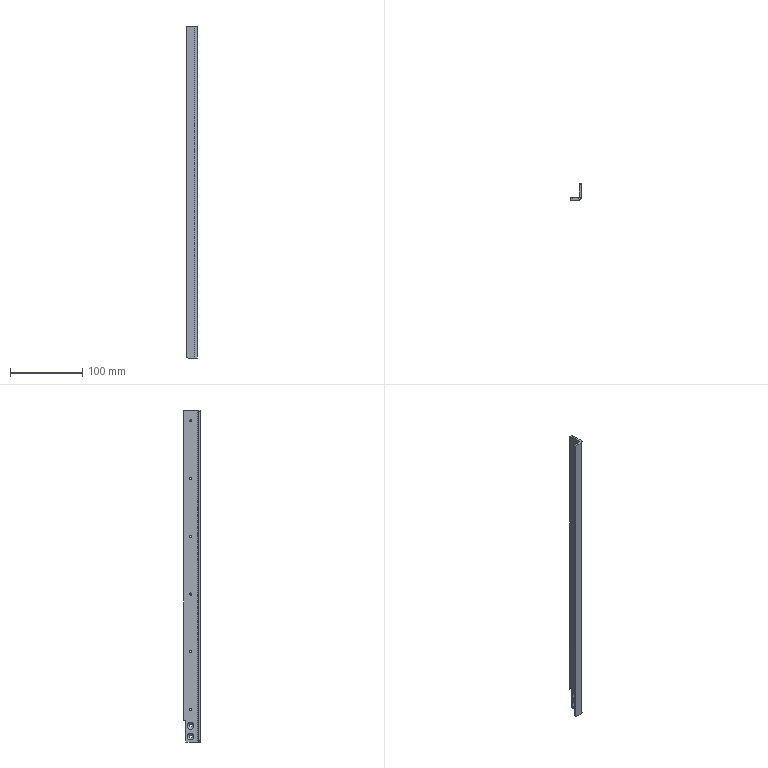Part | NX | features BREP 1 | 1 solid | 51 faces | box 15 x 23 x 460 mm | volume 46240 mm3 | cylinder 21 | cone 16 | plane 14 | commonest cylinder face diameters 2.5 x12 4.5 x4 4 x3 2 x1 8 x1
STEP:
#1=CARTESIAN_POINT('',(-12.,-3.,-228.));
#2=VERTEX_POINT('',#1);
#3=CARTESIAN_POINT('',(-10.,-3.,-230.));
#4=VERTEX_POINT('',#3);
#5=CARTESIAN_POINT('',(-10.,-3.,-228.));
#6=DIRECTION('',(0.,-1.,0.));
#7=DIRECTION('',(-1.,0.,0.));
#8=AXIS2_PLACEMENT_3D('',#5,#6,#7);
#9=CIRCLE('',#8,2.);
#10=EDGE_CURVE('',#2,#4,#9,.T.);
#11=ORIENTED_EDGE('',*,*,#10,.F.);
#12=CARTESIAN_POINT('',(-12.,0.,-228.));
#13=VERTEX_POINT('',#12);
#14=CARTESIAN_POINT('',(-12.,-3.,-228.));
#15=DIRECTION('',(0.,-1.,0.));
#16=VECTOR('',#15,1000.);
#17=LINE('',#14,#16);
#18=EDGE_CURVE('',#13,#2,#17,.T.);
#19=ORIENTED_EDGE('',*,*,#18,.F.);
#20=CARTESIAN_POINT('',(-10.,0.,-230.));
#21=VERTEX_POINT('',#20);
#22=CARTESIAN_POINT('',(-10.,0.,-228.));
#23=DIRECTION('',(0.,1.,0.));
#24=DIRECTION('',(-1.,0.,0.));
#25=AXIS2_PLACEMENT_3D('',#22,#23,#24);
#26=CIRCLE('',#25,2.);
#27=EDGE_CURVE('',#21,#13,#26,.T.);
#28=ORIENTED_EDGE('',*,*,#27,.F.);
#29=CARTESIAN_POINT('',(-10.,1.,-230.));
#30=DIRECTION('',(0.,1.,0.));
#31=VECTOR('',#30,1000.);
#32=LINE('',#29,#31);
#33=EDGE_CURVE('',#4,#21,#32,.T.);
#34=ORIENTED_EDGE('',*,*,#33,.F.);
#35=EDGE_LOOP('',(#11,#19,#28,#34));
#36=FACE_BOUND('',#35,.T.);
#37=CARTESIAN_POINT('',(-10.,1.,-228.));
#38=DIRECTION('',(0.,1.,0.));
#39=DIRECTION('',(0.,0.,1.));
#40=AXIS2_PLACEMENT_3D('',#37,#38,#39);
#41=CYLINDRICAL_SURFACE('',#40,2.);
#42=ADVANCED_FACE('',(#36),#41,.T.);
#43=CARTESIAN_POINT('',(-10.,-3.,230.));
#44=VERTEX_POINT('',#43);
#45=CARTESIAN_POINT('',(-12.,-3.,228.));
#46=VERTEX_POINT('',#45);
#47=CARTESIAN_POINT('',(-10.,-3.,228.));
#48=DIRECTION('',(0.,-1.,0.));
#49=DIRECTION('',(-1.,0.,0.));
#50=AXIS2_PLACEMENT_3D('',#47,#48,#49);
#51=CIRCLE('',#50,2.);
#52=EDGE_CURVE('',#44,#46,#51,.T.);
#53=ORIENTED_EDGE('',*,*,#52,.F.);
#54=CARTESIAN_POINT('',(-10.,0.,230.));
#55=VERTEX_POINT('',#54);
#56=CARTESIAN_POINT('',(-10.,-3.,230.));
#57=DIRECTION('',(0.,-1.,0.));
#58=VECTOR('',#57,1000.);
#59=LINE('',#56,#58);
#60=EDGE_CURVE('',#55,#44,#59,.T.);
#61=ORIENTED_EDGE('',*,*,#60,.F.);
#62=CARTESIAN_POINT('',(-12.,0.,228.));
#63=VERTEX_POINT('',#62);
#64=CARTESIAN_POINT('',(-10.,0.,228.));
#65=DIRECTION('',(0.,1.,0.));
#66=DIRECTION('',(-1.,0.,0.));
#67=AXIS2_PLACEMENT_3D('',#64,#65,#66);
#68=CIRCLE('',#67,2.);
#69=EDGE_CURVE('',#63,#55,#68,.T.);
#70=ORIENTED_EDGE('',*,*,#69,.F.);
#71=CARTESIAN_POINT('',(-12.,0.,228.));
#72=DIRECTION('',(0.,1.,0.));
#73=VECTOR('',#72,1000.);
#74=LINE('',#71,#73);
#75=EDGE_CURVE('',#46,#63,#74,.T.);
#76=ORIENTED_EDGE('',*,*,#75,.F.);
#77=EDGE_LOOP('',(#53,#61,#70,#76));
#78=FACE_BOUND('',#77,.T.);
#79=CARTESIAN_POINT('',(-10.,-3.,228.));
#80=DIRECTION('',(0.,-1.,0.));
#81=DIRECTION('',(0.,0.,-1.));
#82=AXIS2_PLACEMENT_3D('',#79,#80,#81);
#83=CYLINDRICAL_SURFACE('',#82,2.);
#84=ADVANCED_FACE('',(#78),#83,.T.);
#85=CARTESIAN_POINT('',(0.,18.,230.));
#86=VERTEX_POINT('',#85);
#87=CARTESIAN_POINT('',(0.,20.,228.));
#88=VERTEX_POINT('',#87);
#89=CARTESIAN_POINT('',(0.,18.,228.));
#90=DIRECTION('',(-1.,0.,0.));
#91=DIRECTION('',(0.,0.,1.));
#92=AXIS2_PLACEMENT_3D('',#89,#90,#91);
#93=CIRCLE('',#92,2.);
#94=EDGE_CURVE('',#86,#88,#93,.T.);
#95=ORIENTED_EDGE('',*,*,#94,.F.);
#96=CARTESIAN_POINT('',(3.,18.,230.));
#97=VERTEX_POINT('',#96);
#98=CARTESIAN_POINT('',(-1.,18.,230.));
#99=DIRECTION('',(-1.,0.,0.));
#100=VECTOR('',#99,1000.);
#101=LINE('',#98,#100);
#102=EDGE_CURVE('',#97,#86,#101,.T.);
#103=ORIENTED_EDGE('',*,*,#102,.F.);
#104=CARTESIAN_POINT('',(3.,20.,228.));
#105=VERTEX_POINT('',#104);
#106=CARTESIAN_POINT('',(3.,18.,228.));
#107=DIRECTION('',(1.,0.,0.));
#108=DIRECTION('',(0.,0.,1.));
#109=AXIS2_PLACEMENT_3D('',#106,#107,#108);
#110=CIRCLE('',#109,2.);
#111=EDGE_CURVE('',#105,#97,#110,.T.);
#112=ORIENTED_EDGE('',*,*,#111,.F.);
#113=CARTESIAN_POINT('',(0.,20.,228.));
#114=DIRECTION('',(1.,0.,0.));
#115=VECTOR('',#114,1000.);
#116=LINE('',#113,#115);
#117=EDGE_CURVE('',#88,#105,#116,.T.);
#118=ORIENTED_EDGE('',*,*,#117,.F.);
#119=EDGE_LOOP('',(#95,#103,#112,#118));
#120=FACE_BOUND('',#119,.T.);
#121=CARTESIAN_POINT('',(0.,18.,228.));
#122=DIRECTION('',(1.,0.,0.));
#123=DIRECTION('',(0.,0.,-1.));
#124=AXIS2_PLACEMENT_3D('',#121,#122,#123);
#125=CYLINDRICAL_SURFACE('',#124,2.);
#126=ADVANCED_FACE('',(#120),#125,.T.);
#127=CARTESIAN_POINT('',(0.,10.5,213.475));
#128=VERTEX_POINT('',#127);
#129=CARTESIAN_POINT('',(0.275,10.5,213.75));
#130=VERTEX_POINT('',#129);
#131=CARTESIAN_POINT('',(0.,10.5,213.475));
#132=DIRECTION('',(-0.7071,0.,-0.7071));
#133=VECTOR('',#132,1000.);
#134=LINE('',#131,#133);
#135=EDGE_CURVE('',#128,#130,#134,.F.);
#136=ORIENTED_EDGE('',*,*,#135,.T.);
#137=CARTESIAN_POINT('',(0.275,10.5,216.25));
#138=VERTEX_POINT('',#137);
#139=CARTESIAN_POINT('',(0.275,10.5,215.));
#140=DIRECTION('',(-1.,0.,0.));
#141=DIRECTION('',(0.,0.,1.));
#142=AXIS2_PLACEMENT_3D('',#139,#140,#141);
#143=CIRCLE('',#142,1.25);
#144=EDGE_CURVE('',#138,#130,#143,.T.);
#145=ORIENTED_EDGE('',*,*,#144,.F.);
#146=CARTESIAN_POINT('',(0.,10.5,216.525));
#147=VERTEX_POINT('',#146);
#148=CARTESIAN_POINT('',(0.,10.5,216.525));
#149=DIRECTION('',(-0.7071,0.,0.7071));
#150=VECTOR('',#149,1000.);
#151=LINE('',#148,#150);
#152=EDGE_CURVE('',#147,#138,#151,.F.);
#153=ORIENTED_EDGE('',*,*,#152,.F.);
#154=CARTESIAN_POINT('',(0.,10.5,215.));
#155=DIRECTION('',(-1.,0.,0.));
#156=DIRECTION('',(0.,0.,1.));
#157=AXIS2_PLACEMENT_3D('',#154,#155,#156);
#158=CIRCLE('',#157,1.525);
#159=EDGE_CURVE('',#147,#128,#158,.T.);
#160=ORIENTED_EDGE('',*,*,#159,.T.);
#161=EDGE_LOOP('',(#136,#145,#153,#160));
#162=FACE_BOUND('',#161,.T.);
#163=CARTESIAN_POINT('',(0.,10.5,215.));
#164=DIRECTION('',(-1.,0.,0.));
#165=DIRECTION('',(0.,0.,1.));
#166=AXIS2_PLACEMENT_3D('',#163,#164,#165);
#167=CONICAL_SURFACE('',#166,1.525,0.7854);
#168=ADVANCED_FACE('',(#162),#167,.F.);
#169=CARTESIAN_POINT('',(3.,10.5,213.75));
#170=VERTEX_POINT('',#169);
#171=CARTESIAN_POINT('',(0.,10.5,213.75));
#172=DIRECTION('',(-1.,0.,0.));
#173=VECTOR('',#172,1000.);
#174=LINE('',#171,#173);
#175=EDGE_CURVE('',#130,#170,#174,.F.);
#176=ORIENTED_EDGE('',*,*,#175,.T.);
#177=CARTESIAN_POINT('',(3.,10.5,216.25));
#178=VERTEX_POINT('',#177);
#179=CARTESIAN_POINT('',(3.,10.5,215.));
#180=DIRECTION('',(-1.,0.,0.));
#181=DIRECTION('',(0.,0.,1.));
#182=AXIS2_PLACEMENT_3D('',#179,#180,#181);
#183=CIRCLE('',#182,1.25);
#184=EDGE_CURVE('',#178,#170,#183,.T.);
#185=ORIENTED_EDGE('',*,*,#184,.F.);
#186=CARTESIAN_POINT('',(0.,10.5,216.25));
#187=DIRECTION('',(-1.,0.,0.));
#188=VECTOR('',#187,1000.);
#189=LINE('',#186,#188);
#190=EDGE_CURVE('',#138,#178,#189,.F.);
#191=ORIENTED_EDGE('',*,*,#190,.F.);
#192=ORIENTED_EDGE('',*,*,#144,.T.);
#193=EDGE_LOOP('',(#176,#185,#191,#192));
#194=FACE_BOUND('',#193,.T.);
#195=CARTESIAN_POINT('',(0.,10.5,215.));
#196=DIRECTION('',(-1.,0.,0.));
#197=DIRECTION('',(0.,0.,1.));
#198=AXIS2_PLACEMENT_3D('',#195,#196,#197);
#199=CYLINDRICAL_SURFACE('',#198,1.25);
#200=ADVANCED_FACE('',(#194),#199,.F.);
#201=CARTESIAN_POINT('',(0.,10.5,133.475));
#202=VERTEX_POINT('',#201);
#203=CARTESIAN_POINT('',(0.275,10.5,133.75));
#204=VERTEX_POINT('',#203);
#205=CARTESIAN_POINT('',(0.,10.5,133.475));
#206=DIRECTION('',(-0.7071,0.,-0.7071));
#207=VECTOR('',#206,1000.);
#208=LINE('',#205,#207);
#209=EDGE_CURVE('',#202,#204,#208,.F.);
#210=ORIENTED_EDGE('',*,*,#209,.T.);
#211=CARTESIAN_POINT('',(0.275,10.5,136.25));
#212=VERTEX_POINT('',#211);
#213=CARTESIAN_POINT('',(0.275,10.5,135.));
#214=DIRECTION('',(-1.,0.,0.));
#215=DIRECTION('',(0.,0.,1.));
#216=AXIS2_PLACEMENT_3D('',#213,#214,#215);
#217=CIRCLE('',#216,1.25);
#218=EDGE_CURVE('',#212,#204,#217,.T.);
#219=ORIENTED_EDGE('',*,*,#218,.F.);
#220=CARTESIAN_POINT('',(0.,10.5,136.525));
#221=VERTEX_POINT('',#220);
#222=CARTESIAN_POINT('',(0.,10.5,136.525));
#223=DIRECTION('',(-0.7071,0.,0.7071));
#224=VECTOR('',#223,1000.);
#225=LINE('',#222,#224);
#226=EDGE_CURVE('',#221,#212,#225,.F.);
#227=ORIENTED_EDGE('',*,*,#226,.F.);
#228=CARTESIAN_POINT('',(0.,10.5,135.));
#229=DIRECTION('',(-1.,0.,0.));
#230=DIRECTION('',(0.,0.,1.));
#231=AXIS2_PLACEMENT_3D('',#228,#229,#230);
#232=CIRCLE('',#231,1.525);
#233=EDGE_CURVE('',#221,#202,#232,.T.);
#234=ORIENTED_EDGE('',*,*,#233,.T.);
#235=EDGE_LOOP('',(#210,#219,#227,#234));
#236=FACE_BOUND('',#235,.T.);
#237=CARTESIAN_POINT('',(0.,10.5,135.));
#238=DIRECTION('',(-1.,0.,0.));
#239=DIRECTION('',(0.,0.,1.));
#240=AXIS2_PLACEMENT_3D('',#237,#238,#239);
#241=CONICAL_SURFACE('',#240,1.525,0.7854);
#242=ADVANCED_FACE('',(#236),#241,.F.);
#243=CARTESIAN_POINT('',(3.,10.5,133.75));
#244=VERTEX_POINT('',#243);
#245=CARTESIAN_POINT('',(0.,10.5,133.75));
#246=DIRECTION('',(-1.,0.,0.));
#247=VECTOR('',#246,1000.);
#248=LINE('',#245,#247);
#249=EDGE_CURVE('',#204,#244,#248,.F.);
#250=ORIENTED_EDGE('',*,*,#249,.T.);
#251=CARTESIAN_POINT('',(3.,10.5,136.25));
#252=VERTEX_POINT('',#251);
#253=CARTESIAN_POINT('',(3.,10.5,135.));
#254=DIRECTION('',(-1.,0.,0.));
#255=DIRECTION('',(0.,0.,1.));
#256=AXIS2_PLACEMENT_3D('',#253,#254,#255);
#257=CIRCLE('',#256,1.25);
#258=EDGE_CURVE('',#252,#244,#257,.T.);
#259=ORIENTED_EDGE('',*,*,#258,.F.);
#260=CARTESIAN_POINT('',(0.,10.5,136.25));
#261=DIRECTION('',(-1.,0.,0.));
#262=VECTOR('',#261,1000.);
#263=LINE('',#260,#262);
#264=EDGE_CURVE('',#212,#252,#263,.F.);
#265=ORIENTED_EDGE('',*,*,#264,.F.);
#266=ORIENTED_EDGE('',*,*,#218,.T.);
#267=EDGE_LOOP('',(#250,#259,#265,#266));
#268=FACE_BOUND('',#267,.T.);
#269=CARTESIAN_POINT('',(0.,10.5,135.));
#270=DIRECTION('',(-1.,0.,0.));
#271=DIRECTION('',(0.,0.,1.));
#272=AXIS2_PLACEMENT_3D('',#269,#270,#271);
#273=CYLINDRICAL_SURFACE('',#272,1.25);
#274=ADVANCED_FACE('',(#268),#273,.F.);
#275=CARTESIAN_POINT('',(0.,10.5,53.475));
#276=VERTEX_POINT('',#275);
#277=CARTESIAN_POINT('',(0.275,10.5,53.75));
#278=VERTEX_POINT('',#277);
#279=CARTESIAN_POINT('',(0.,10.5,53.475));
#280=DIRECTION('',(-0.7071,0.,-0.7071));
#281=VECTOR('',#280,1000.);
#282=LINE('',#279,#281);
#283=EDGE_CURVE('',#276,#278,#282,.F.);
#284=ORIENTED_EDGE('',*,*,#283,.T.);
#285=CARTESIAN_POINT('',(0.275,10.5,56.25));
#286=VERTEX_POINT('',#285);
#287=CARTESIAN_POINT('',(0.275,10.5,55.));
#288=DIRECTION('',(-1.,0.,0.));
#289=DIRECTION('',(0.,0.,1.));
#290=AXIS2_PLACEMENT_3D('',#287,#288,#289);
#291=CIRCLE('',#290,1.25);
#292=EDGE_CURVE('',#286,#278,#291,.T.);
#293=ORIENTED_EDGE('',*,*,#292,.F.);
#294=CARTESIAN_POINT('',(0.,10.5,56.525));
#295=VERTEX_POINT('',#294);
#296=CARTESIAN_POINT('',(0.,10.5,56.525));
#297=DIRECTION('',(-0.7071,0.,0.7071));
#298=VECTOR('',#297,1000.);
#299=LINE('',#296,#298);
#300=EDGE_CURVE('',#295,#286,#299,.F.);
#301=ORIENTED_EDGE('',*,*,#300,.F.);
#302=CARTESIAN_POINT('',(0.,10.5,55.));
#303=DIRECTION('',(-1.,0.,0.));
#304=DIRECTION('',(0.,0.,1.));
#305=AXIS2_PLACEMENT_3D('',#302,#303,#304);
#306=CIRCLE('',#305,1.525);
#307=EDGE_CURVE('',#295,#276,#306,.T.);
#308=ORIENTED_EDGE('',*,*,#307,.T.);
#309=EDGE_LOOP('',(#284,#293,#301,#308));
#310=FACE_BOUND('',#309,.T.);
#311=CARTESIAN_POINT('',(0.,10.5,55.));
#312=DIRECTION('',(-1.,0.,0.));
#313=DIRECTION('',(0.,0.,1.));
#314=AXIS2_PLACEMENT_3D('',#311,#312,#313);
#315=CONICAL_SURFACE('',#314,1.525,0.7854);
#316=ADVANCED_FACE('',(#310),#315,.F.);
#317=CARTESIAN_POINT('',(3.,10.5,53.75));
#318=VERTEX_POINT('',#317);
#319=CARTESIAN_POINT('',(0.,10.5,53.75));
#320=DIRECTION('',(-1.,0.,0.));
#321=VECTOR('',#320,1000.);
#322=LINE('',#319,#321);
#323=EDGE_CURVE('',#278,#318,#322,.F.);
#324=ORIENTED_EDGE('',*,*,#323,.T.);
#325=CARTESIAN_POINT('',(3.,10.5,56.25));
#326=VERTEX_POINT('',#325);
#327=CARTESIAN_POINT('',(3.,10.5,55.));
#328=DIRECTION('',(-1.,0.,0.));
#329=DIRECTION('',(0.,0.,1.));
#330=AXIS2_PLACEMENT_3D('',#327,#328,#329);
#331=CIRCLE('',#330,1.25);
#332=EDGE_CURVE('',#326,#318,#331,.T.);
#333=ORIENTED_EDGE('',*,*,#332,.F.);
#334=CARTESIAN_POINT('',(0.,10.5,56.25));
#335=DIRECTION('',(-1.,0.,0.));
#336=VECTOR('',#335,1000.);
#337=LINE('',#334,#336);
#338=EDGE_CURVE('',#286,#326,#337,.F.);
#339=ORIENTED_EDGE('',*,*,#338,.F.);
#340=ORIENTED_EDGE('',*,*,#292,.T.);
#341=EDGE_LOOP('',(#324,#333,#339,#340));
#342=FACE_BOUND('',#341,.T.);
#343=CARTESIAN_POINT('',(0.,10.5,55.));
#344=DIRECTION('',(-1.,0.,0.));
#345=DIRECTION('',(0.,0.,1.));
#346=AXIS2_PLACEMENT_3D('',#343,#344,#345);
#347=CYLINDRICAL_SURFACE('',#346,1.25);
#348=ADVANCED_FACE('',(#342),#347,.F.);
#349=CARTESIAN_POINT('',(0.,10.5,-26.525));
#350=VERTEX_POINT('',#349);
#351=CARTESIAN_POINT('',(0.275,10.5,-26.25));
#352=VERTEX_POINT('',#351);
#353=CARTESIAN_POINT('',(0.,10.5,-26.525));
#354=DIRECTION('',(-0.7071,0.,-0.7071));
#355=VECTOR('',#354,1000.);
#356=LINE('',#353,#355);
#357=EDGE_CURVE('',#350,#352,#356,.F.);
#358=ORIENTED_EDGE('',*,*,#357,.T.);
#359=CARTESIAN_POINT('',(0.275,10.5,-23.75));
#360=VERTEX_POINT('',#359);
#361=CARTESIAN_POINT('',(0.275,10.5,-25.));
#362=DIRECTION('',(-1.,0.,0.));
#363=DIRECTION('',(0.,0.,1.));
#364=AXIS2_PLACEMENT_3D('',#361,#362,#363);
#365=CIRCLE('',#364,1.25);
#366=EDGE_CURVE('',#360,#352,#365,.T.);
#367=ORIENTED_EDGE('',*,*,#366,.F.);
#368=CARTESIAN_POINT('',(0.,10.5,-23.475));
#369=VERTEX_POINT('',#368);
#370=CARTESIAN_POINT('',(0.,10.5,-23.475));
#371=DIRECTION('',(-0.7071,0.,0.7071));
#372=VECTOR('',#371,1000.);
#373=LINE('',#370,#372);
#374=EDGE_CURVE('',#369,#360,#373,.F.);
#375=ORIENTED_EDGE('',*,*,#374,.F.);
#376=CARTESIAN_POINT('',(0.,10.5,-25.));
#377=DIRECTION('',(-1.,0.,0.));
#378=DIRECTION('',(0.,0.,1.));
#379=AXIS2_PLACEMENT_3D('',#376,#377,#378);
#380=CIRCLE('',#379,1.525);
#381=EDGE_CURVE('',#369,#350,#380,.T.);
#382=ORIENTED_EDGE('',*,*,#381,.T.);
#383=EDGE_LOOP('',(#358,#367,#375,#382));
#384=FACE_BOUND('',#383,.T.);
#385=CARTESIAN_POINT('',(0.,10.5,-25.));
#386=DIRECTION('',(-1.,0.,0.));
#387=DIRECTION('',(0.,0.,1.));
#388=AXIS2_PLACEMENT_3D('',#385,#386,#387);
#389=CONICAL_SURFACE('',#388,1.525,0.7854);
#390=ADVANCED_FACE('',(#384),#389,.F.);
#391=CARTESIAN_POINT('',(3.,10.5,-26.25));
#392=VERTEX_POINT('',#391);
#393=CARTESIAN_POINT('',(0.,10.5,-26.25));
#394=DIRECTION('',(-1.,0.,0.));
#395=VECTOR('',#394,1000.);
#396=LINE('',#393,#395);
#397=EDGE_CURVE('',#352,#392,#396,.F.);
#398=ORIENTED_EDGE('',*,*,#397,.T.);
#399=CARTESIAN_POINT('',(3.,10.5,-23.75));
#400=VERTEX_POINT('',#399);
#401=CARTESIAN_POINT('',(3.,10.5,-25.));
#402=DIRECTION('',(-1.,0.,0.));
#403=DIRECTION('',(0.,0.,1.));
#404=AXIS2_PLACEMENT_3D('',#401,#402,#403);
#405=CIRCLE('',#404,1.25);
#406=EDGE_CURVE('',#400,#392,#405,.T.);
#407=ORIENTED_EDGE('',*,*,#406,.F.);
#408=CARTESIAN_POINT('',(0.,10.5,-23.75));
#409=DIRECTION('',(-1.,0.,0.));
#410=VECTOR('',#409,1000.);
#411=LINE('',#408,#410);
#412=EDGE_CURVE('',#360,#400,#411,.F.);
#413=ORIENTED_EDGE('',*,*,#412,.F.);
#414=ORIENTED_EDGE('',*,*,#366,.T.);
#415=EDGE_LOOP('',(#398,#407,#413,#414));
#416=FACE_BOUND('',#415,.T.);
#417=CARTESIAN_POINT('',(0.,10.5,-25.));
#418=DIRECTION('',(-1.,0.,0.));
#419=DIRECTION('',(0.,0.,1.));
#420=AXIS2_PLACEMENT_3D('',#417,#418,#419);
#421=CYLINDRICAL_SURFACE('',#420,1.25);
#422=ADVANCED_FACE('',(#416),#421,.F.);
#423=CARTESIAN_POINT('',(0.,10.5,-106.525));
#424=VERTEX_POINT('',#423);
#425=CARTESIAN_POINT('',(0.275,10.5,-106.25));
#426=VERTEX_POINT('',#425);
#427=CARTESIAN_POINT('',(0.,10.5,-106.525));
#428=DIRECTION('',(-0.7071,0.,-0.7071));
#429=VECTOR('',#428,1000.);
#430=LINE('',#427,#429);
#431=EDGE_CURVE('',#424,#426,#430,.F.);
#432=ORIENTED_EDGE('',*,*,#431,.T.);
#433=CARTESIAN_POINT('',(0.275,10.5,-103.75));
#434=VERTEX_POINT('',#433);
#435=CARTESIAN_POINT('',(0.275,10.5,-105.));
#436=DIRECTION('',(-1.,0.,0.));
#437=DIRECTION('',(0.,0.,1.));
#438=AXIS2_PLACEMENT_3D('',#435,#436,#437);
#439=CIRCLE('',#438,1.25);
#440=EDGE_CURVE('',#434,#426,#439,.T.);
#441=ORIENTED_EDGE('',*,*,#440,.F.);
#442=CARTESIAN_POINT('',(0.,10.5,-103.475));
#443=VERTEX_POINT('',#442);
#444=CARTESIAN_POINT('',(0.,10.5,-103.475));
#445=DIRECTION('',(-0.7071,0.,0.7071));
#446=VECTOR('',#445,1000.);
#447=LINE('',#444,#446);
#448=EDGE_CURVE('',#443,#434,#447,.F.);
#449=ORIENTED_EDGE('',*,*,#448,.F.);
#450=CARTESIAN_POINT('',(0.,10.5,-105.));
#451=DIRECTION('',(-1.,0.,0.));
#452=DIRECTION('',(0.,0.,1.));
#453=AXIS2_PLACEMENT_3D('',#450,#451,#452);
#454=CIRCLE('',#453,1.525);
#455=EDGE_CURVE('',#443,#424,#454,.T.);
#456=ORIENTED_EDGE('',*,*,#455,.T.);
#457=EDGE_LOOP('',(#432,#441,#449,#456));
#458=FACE_BOUND('',#457,.T.);
#459=CARTESIAN_POINT('',(0.,10.5,-105.));
#460=DIRECTION('',(-1.,0.,0.));
#461=DIRECTION('',(0.,0.,1.));
#462=AXIS2_PLACEMENT_3D('',#459,#460,#461);
#463=CONICAL_SURFACE('',#462,1.525,0.7854);
#464=ADVANCED_FACE('',(#458),#463,.F.);
#465=CARTESIAN_POINT('',(3.,10.5,-106.25));
#466=VERTEX_POINT('',#465);
#467=CARTESIAN_POINT('',(0.,10.5,-106.25));
#468=DIRECTION('',(-1.,0.,0.));
#469=VECTOR('',#468,1000.);
#470=LINE('',#467,#469);
#471=EDGE_CURVE('',#426,#466,#470,.F.);
#472=ORIENTED_EDGE('',*,*,#471,.T.);
#473=CARTESIAN_POINT('',(3.,10.5,-103.75));
#474=VERTEX_POINT('',#473);
#475=CARTESIAN_POINT('',(3.,10.5,-105.));
#476=DIRECTION('',(-1.,0.,0.));
#477=DIRECTION('',(0.,0.,1.));
#478=AXIS2_PLACEMENT_3D('',#475,#476,#477);
#479=CIRCLE('',#478,1.25);
#480=EDGE_CURVE('',#474,#466,#479,.T.);
#481=ORIENTED_EDGE('',*,*,#480,.F.);
#482=CARTESIAN_POINT('',(0.,10.5,-103.75));
#483=DIRECTION('',(-1.,0.,0.));
#484=VECTOR('',#483,1000.);
#485=LINE('',#482,#484);
#486=EDGE_CURVE('',#434,#474,#485,.F.);
#487=ORIENTED_EDGE('',*,*,#486,.F.);
#488=ORIENTED_EDGE('',*,*,#440,.T.);
#489=EDGE_LOOP('',(#472,#481,#487,#488));
#490=FACE_BOUND('',#489,.T.);
#491=CARTESIAN_POINT('',(0.,10.5,-105.));
#492=DIRECTION('',(-1.,0.,0.));
#493=DIRECTION('',(0.,0.,1.));
#494=AXIS2_PLACEMENT_3D('',#491,#492,#493);
#495=CYLINDRICAL_SURFACE('',#494,1.25);
#496=ADVANCED_FACE('',(#490),#495,.F.);
#497=CARTESIAN_POINT('',(0.,10.5,-186.525));
#498=VERTEX_POINT('',#497);
#499=CARTESIAN_POINT('',(0.275,10.5,-186.25));
#500=VERTEX_POINT('',#499);
#501=CARTESIAN_POINT('',(0.,10.5,-186.525));
#502=DIRECTION('',(-0.7071,0.,-0.7071));
#503=VECTOR('',#502,1000.);
#504=LINE('',#501,#503);
#505=EDGE_CURVE('',#498,#500,#504,.F.);
#506=ORIENTED_EDGE('',*,*,#505,.T.);
#507=CARTESIAN_POINT('',(0.275,10.5,-183.75));
#508=VERTEX_POINT('',#507);
#509=CARTESIAN_POINT('',(0.275,10.5,-185.));
#510=DIRECTION('',(-1.,0.,0.));
#511=DIRECTION('',(0.,0.,1.));
#512=AXIS2_PLACEMENT_3D('',#509,#510,#511);
#513=CIRCLE('',#512,1.25);
#514=EDGE_CURVE('',#508,#500,#513,.T.);
#515=ORIENTED_EDGE('',*,*,#514,.F.);
#516=CARTESIAN_POINT('',(0.,10.5,-183.475));
#517=VERTEX_POINT('',#516);
#518=CARTESIAN_POINT('',(0.,10.5,-183.475));
#519=DIRECTION('',(-0.7071,0.,0.7071));
#520=VECTOR('',#519,1000.);
#521=LINE('',#518,#520);
#522=EDGE_CURVE('',#517,#508,#521,.F.);
#523=ORIENTED_EDGE('',*,*,#522,.F.);
#524=CARTESIAN_POINT('',(0.,10.5,-185.));
#525=DIRECTION('',(-1.,0.,0.));
#526=DIRECTION('',(0.,0.,1.));
#527=AXIS2_PLACEMENT_3D('',#524,#525,#526);
#528=CIRCLE('',#527,1.525);
#529=EDGE_CURVE('',#517,#498,#528,.T.);
#530=ORIENTED_EDGE('',*,*,#529,.T.);
#531=EDGE_LOOP('',(#506,#515,#523,#530));
#532=FACE_BOUND('',#531,.T.);
#533=CARTESIAN_POINT('',(0.,10.5,-185.));
#534=DIRECTION('',(-1.,0.,0.));
#535=DIRECTION('',(0.,0.,1.));
#536=AXIS2_PLACEMENT_3D('',#533,#534,#535);
#537=CONICAL_SURFACE('',#536,1.525,0.7854);
#538=ADVANCED_FACE('',(#532),#537,.F.);
#539=CARTESIAN_POINT('',(3.,10.5,-186.25));
#540=VERTEX_POINT('',#539);
#541=CARTESIAN_POINT('',(0.,10.5,-186.25));
#542=DIRECTION('',(-1.,0.,0.));
#543=VECTOR('',#542,1000.);
#544=LINE('',#541,#543);
#545=EDGE_CURVE('',#500,#540,#544,.F.);
#546=ORIENTED_EDGE('',*,*,#545,.T.);
#547=CARTESIAN_POINT('',(3.,10.5,-183.75));
#548=VERTEX_POINT('',#547);
#549=CARTESIAN_POINT('',(3.,10.5,-185.));
#550=DIRECTION('',(-1.,0.,0.));
#551=DIRECTION('',(0.,0.,1.));
#552=AXIS2_PLACEMENT_3D('',#549,#550,#551);
#553=CIRCLE('',#552,1.25);
#554=EDGE_CURVE('',#548,#540,#553,.T.);
#555=ORIENTED_EDGE('',*,*,#554,.F.);
#556=CARTESIAN_POINT('',(0.,10.5,-183.75));
#557=DIRECTION('',(-1.,0.,0.));
#558=VECTOR('',#557,1000.);
#559=LINE('',#556,#558);
#560=EDGE_CURVE('',#508,#548,#559,.F.);
#561=ORIENTED_EDGE('',*,*,#560,.F.);
#562=ORIENTED_EDGE('',*,*,#514,.T.);
#563=EDGE_LOOP('',(#546,#555,#561,#562));
#564=FACE_BOUND('',#563,.T.);
#565=CARTESIAN_POINT('',(0.,10.5,-185.));
#566=DIRECTION('',(-1.,0.,0.));
#567=DIRECTION('',(0.,0.,1.));
#568=AXIS2_PLACEMENT_3D('',#565,#566,#567);
#569=CYLINDRICAL_SURFACE('',#568,1.25);
#570=ADVANCED_FACE('',(#564),#569,.F.);
#571=CARTESIAN_POINT('',(0.,10.5,-227.2));
#572=VERTEX_POINT('',#571);
#573=CARTESIAN_POINT('',(2.45,10.5,-224.75));
#574=VERTEX_POINT('',#573);
#575=CARTESIAN_POINT('',(0.,10.5,-227.2));
#576=DIRECTION('',(-0.7071,0.,-0.7071));
#577=VECTOR('',#576,1000.);
#578=LINE('',#575,#577);
#579=EDGE_CURVE('',#572,#574,#578,.F.);
#580=ORIENTED_EDGE('',*,*,#579,.T.);
#581=CARTESIAN_POINT('',(2.45,10.5,-220.25));
#582=VERTEX_POINT('',#581);
#583=CARTESIAN_POINT('',(2.45,10.5,-222.5));
#584=DIRECTION('',(-1.,0.,0.));
#585=DIRECTION('',(0.,0.,1.));
#586=AXIS2_PLACEMENT_3D('',#583,#584,#585);
#587=CIRCLE('',#586,2.25);
#588=EDGE_CURVE('',#582,#574,#587,.T.);
#589=ORIENTED_EDGE('',*,*,#588,.F.);
#590=CARTESIAN_POINT('',(0.,10.5,-217.8));
#591=VERTEX_POINT('',#590);
#592=CARTESIAN_POINT('',(0.,10.5,-217.8));
#593=DIRECTION('',(-0.7071,0.,0.7071));
#594=VECTOR('',#593,1000.);
#595=LINE('',#592,#594);
#596=EDGE_CURVE('',#591,#582,#595,.F.);
#597=ORIENTED_EDGE('',*,*,#596,.F.);
#598=CARTESIAN_POINT('',(0.,10.5,-222.5));
#599=DIRECTION('',(-1.,0.,0.));
#600=DIRECTION('',(0.,0.,1.));
#601=AXIS2_PLACEMENT_3D('',#598,#599,#600);
#602=CIRCLE('',#601,4.7);
#603=EDGE_CURVE('',#591,#572,#602,.T.);
#604=ORIENTED_EDGE('',*,*,#603,.T.);
#605=EDGE_LOOP('',(#580,#589,#597,#604));
#606=FACE_BOUND('',#605,.T.);
#607=CARTESIAN_POINT('',(0.,10.5,-222.5));
#608=DIRECTION('',(-1.,0.,0.));
#609=DIRECTION('',(0.,0.,1.));
#610=AXIS2_PLACEMENT_3D('',#607,#608,#609);
#611=CONICAL_SURFACE('',#610,4.7,0.7854);
#612=ADVANCED_FACE('',(#606),#611,.F.);
#613=CARTESIAN_POINT('',(3.,10.5,-224.75));
#614=VERTEX_POINT('',#613);
#615=CARTESIAN_POINT('',(0.,10.5,-224.75));
#616=DIRECTION('',(-1.,0.,0.));
#617=VECTOR('',#616,1000.);
#618=LINE('',#615,#617);
#619=EDGE_CURVE('',#574,#614,#618,.F.);
#620=ORIENTED_EDGE('',*,*,#619,.T.);
#621=CARTESIAN_POINT('',(3.,10.5,-220.25));
#622=VERTEX_POINT('',#621);
#623=CARTESIAN_POINT('',(3.,10.5,-222.5));
#624=DIRECTION('',(-1.,0.,0.));
#625=DIRECTION('',(0.,0.,1.));
#626=AXIS2_PLACEMENT_3D('',#623,#624,#625);
#627=CIRCLE('',#626,2.25);
#628=EDGE_CURVE('',#622,#614,#627,.T.);
#629=ORIENTED_EDGE('',*,*,#628,.F.);
#630=CARTESIAN_POINT('',(0.,10.5,-220.25));
#631=DIRECTION('',(-1.,0.,0.));
#632=VECTOR('',#631,1000.);
#633=LINE('',#630,#632);
#634=EDGE_CURVE('',#582,#622,#633,.F.);
#635=ORIENTED_EDGE('',*,*,#634,.F.);
#636=ORIENTED_EDGE('',*,*,#588,.T.);
#637=EDGE_LOOP('',(#620,#629,#635,#636));
#638=FACE_BOUND('',#637,.T.);
#639=CARTESIAN_POINT('',(0.,10.5,-222.5));
#640=DIRECTION('',(-1.,0.,0.));
#641=DIRECTION('',(0.,0.,1.));
#642=AXIS2_PLACEMENT_3D('',#639,#640,#641);
#643=CYLINDRICAL_SURFACE('',#642,2.25);
#644=ADVANCED_FACE('',(#638),#643,.F.);
#645=CARTESIAN_POINT('',(0.,10.5,-212.2));
#646=VERTEX_POINT('',#645);
#647=CARTESIAN_POINT('',(2.45,10.5,-209.75));
#648=VERTEX_POINT('',#647);
#649=CARTESIAN_POINT('',(0.,10.5,-212.2));
#650=DIRECTION('',(-0.7071,0.,-0.7071));
#651=VECTOR('',#650,1000.);
#652=LINE('',#649,#651);
#653=EDGE_CURVE('',#646,#648,#652,.F.);
#654=ORIENTED_EDGE('',*,*,#653,.T.);
#655=CARTESIAN_POINT('',(2.45,10.5,-205.25));
#656=VERTEX_POINT('',#655);
#657=CARTESIAN_POINT('',(2.45,10.5,-207.5));
#658=DIRECTION('',(-1.,0.,0.));
#659=DIRECTION('',(0.,0.,1.));
#660=AXIS2_PLACEMENT_3D('',#657,#658,#659);
#661=CIRCLE('',#660,2.25);
#662=EDGE_CURVE('',#656,#648,#661,.T.);
#663=ORIENTED_EDGE('',*,*,#662,.F.);
#664=CARTESIAN_POINT('',(0.,10.5,-202.8));
#665=VERTEX_POINT('',#664);
#666=CARTESIAN_POINT('',(0.,10.5,-202.8));
#667=DIRECTION('',(-0.7071,0.,0.7071));
#668=VECTOR('',#667,1000.);
#669=LINE('',#666,#668);
#670=EDGE_CURVE('',#665,#656,#669,.F.);
#671=ORIENTED_EDGE('',*,*,#670,.F.);
#672=CARTESIAN_POINT('',(0.,10.5,-207.5));
#673=DIRECTION('',(-1.,0.,0.));
#674=DIRECTION('',(0.,0.,1.));
#675=AXIS2_PLACEMENT_3D('',#672,#673,#674);
#676=CIRCLE('',#675,4.7);
#677=EDGE_CURVE('',#665,#646,#676,.T.);
#678=ORIENTED_EDGE('',*,*,#677,.T.);
#679=EDGE_LOOP('',(#654,#663,#671,#678));
#680=FACE_BOUND('',#679,.T.);
#681=CARTESIAN_POINT('',(0.,10.5,-207.5));
#682=DIRECTION('',(-1.,0.,0.));
#683=DIRECTION('',(0.,0.,1.));
#684=AXIS2_PLACEMENT_3D('',#681,#682,#683);
#685=CONICAL_SURFACE('',#684,4.7,0.7854);
#686=ADVANCED_FACE('',(#680),#685,.F.);
#687=CARTESIAN_POINT('',(3.,10.5,-209.75));
#688=VERTEX_POINT('',#687);
#689=CARTESIAN_POINT('',(0.,10.5,-209.75));
#690=DIRECTION('',(-1.,0.,0.));
#691=VECTOR('',#690,1000.);
#692=LINE('',#689,#691);
#693=EDGE_CURVE('',#648,#688,#692,.F.);
#694=ORIENTED_EDGE('',*,*,#693,.T.);
#695=CARTESIAN_POINT('',(3.,10.5,-205.25));
#696=VERTEX_POINT('',#695);
#697=CARTESIAN_POINT('',(3.,10.5,-207.5));
#698=DIRECTION('',(-1.,0.,0.));
#699=DIRECTION('',(0.,0.,1.));
#700=AXIS2_PLACEMENT_3D('',#697,#698,#699);
#701=CIRCLE('',#700,2.25);
#702=EDGE_CURVE('',#696,#688,#701,.T.);
#703=ORIENTED_EDGE('',*,*,#702,.F.);
#704=CARTESIAN_POINT('',(0.,10.5,-205.25));
#705=DIRECTION('',(-1.,0.,0.));
#706=VECTOR('',#705,1000.);
#707=LINE('',#704,#706);
#708=EDGE_CURVE('',#656,#696,#707,.F.);
#709=ORIENTED_EDGE('',*,*,#708,.F.);
#710=ORIENTED_EDGE('',*,*,#662,.T.);
#711=EDGE_LOOP('',(#694,#703,#709,#710));
#712=FACE_BOUND('',#711,.T.);
#713=CARTESIAN_POINT('',(0.,10.5,-207.5));
#714=DIRECTION('',(-1.,0.,0.));
#715=DIRECTION('',(0.,0.,1.));
#716=AXIS2_PLACEMENT_3D('',#713,#714,#715);
#717=CYLINDRICAL_SURFACE('',#716,2.25);
#718=ADVANCED_FACE('',(#712),#717,.F.);
#719=CARTESIAN_POINT('',(0.,17.,-200.));
#720=VERTEX_POINT('',#719);
#721=CARTESIAN_POINT('',(0.,20.,-200.));
#722=VERTEX_POINT('',#721);
#723=CARTESIAN_POINT('',(0.,0.,-200.));
#724=DIRECTION('',(0.,1.,0.));
#725=VECTOR('',#724,1000.);
#726=LINE('',#723,#725);
#727=EDGE_CURVE('',#720,#722,#726,.T.);
#728=ORIENTED_EDGE('',*,*,#727,.T.);
#729=CARTESIAN_POINT('',(3.,20.,-200.));
#730=VERTEX_POINT('',#729);
#731=CARTESIAN_POINT('',(-7.,20.,-200.));
#732=DIRECTION('',(1.,0.,0.));
#733=VECTOR('',#732,1000.);
#734=LINE('',#731,#733);
#735=EDGE_CURVE('',#722,#730,#734,.T.);
#736=ORIENTED_EDGE('',*,*,#735,.T.);
#737=CARTESIAN_POINT('',(3.,17.,-200.));
#738=VERTEX_POINT('',#737);
#739=CARTESIAN_POINT('',(3.,20.,-200.));
#740=DIRECTION('',(0.,-1.,0.));
#741=VECTOR('',#740,1000.);
#742=LINE('',#739,#741);
#743=EDGE_CURVE('',#730,#738,#742,.T.);
#744=ORIENTED_EDGE('',*,*,#743,.T.);
#745=CARTESIAN_POINT('',(-7.,17.,-200.));
#746=DIRECTION('',(1.,0.,0.));
#747=VECTOR('',#746,1000.);
#748=LINE('',#745,#747);
#749=EDGE_CURVE('',#720,#738,#748,.T.);
#750=ORIENTED_EDGE('',*,*,#749,.F.);
#751=EDGE_LOOP('',(#728,#736,#744,#750));
#752=FACE_BOUND('',#751,.T.);
#753=CARTESIAN_POINT('',(-7.,20.,-200.));
#754=DIRECTION('',(0.,0.,1.));
#755=DIRECTION('',(1.,0.,0.));
#756=AXIS2_PLACEMENT_3D('',#753,#754,#755);
#757=PLANE('',#756);
#758=ADVANCED_FACE('',(#752),#757,.F.);
#759=CARTESIAN_POINT('',(0.,17.,-230.));
#760=VERTEX_POINT('',#759);
#761=CARTESIAN_POINT('',(0.,17.,230.));
#762=DIRECTION('',(0.,0.,1.));
#763=VECTOR('',#762,1000.);
#764=LINE('',#761,#763);
#765=EDGE_CURVE('',#760,#720,#764,.T.);
#766=ORIENTED_EDGE('',*,*,#765,.T.);
#767=ORIENTED_EDGE('',*,*,#749,.T.);
#768=CARTESIAN_POINT('',(3.,17.,-230.));
#769=VERTEX_POINT('',#768);
#770=CARTESIAN_POINT('',(3.,17.,-230.));
#771=DIRECTION('',(0.,0.,-1.));
#772=VECTOR('',#771,1000.);
#773=LINE('',#770,#772);
#774=EDGE_CURVE('',#738,#769,#773,.T.);
#775=ORIENTED_EDGE('',*,*,#774,.T.);
#776=CARTESIAN_POINT('',(-1.,17.,-230.));
#777=DIRECTION('',(-1.,0.,0.));
#778=VECTOR('',#777,1000.);
#779=LINE('',#776,#778);
#780=EDGE_CURVE('',#769,#760,#779,.T.);
#781=ORIENTED_EDGE('',*,*,#780,.T.);
#782=EDGE_LOOP('',(#766,#767,#775,#781));
#783=FACE_BOUND('',#782,.T.);
#784=CARTESIAN_POINT('',(-7.,17.,-230.));
#785=DIRECTION('',(0.,-1.,0.));
#786=DIRECTION('',(0.,0.,-1.));
#787=AXIS2_PLACEMENT_3D('',#784,#785,#786);
#788=PLANE('',#787);
#789=ADVANCED_FACE('',(#783),#788,.F.);
#790=ORIENTED_EDGE('',*,*,#780,.F.);
#791=CARTESIAN_POINT('',(3.,1.,-230.));
#792=VERTEX_POINT('',#791);
#793=CARTESIAN_POINT('',(3.,0.,-230.));
#794=DIRECTION('',(0.,1.,0.));
#795=VECTOR('',#794,1000.);
#796=LINE('',#793,#795);
#797=EDGE_CURVE('',#792,#769,#796,.T.);
#798=ORIENTED_EDGE('',*,*,#797,.F.);
#799=CARTESIAN_POINT('',(0.,1.,-230.));
#800=VERTEX_POINT('',#799);
#801=CARTESIAN_POINT('',(3.,1.,-230.));
#802=DIRECTION('',(-1.,0.,0.));
#803=VECTOR('',#802,1000.);
#804=LINE('',#801,#803);
#805=EDGE_CURVE('',#792,#800,#804,.T.);
#806=ORIENTED_EDGE('',*,*,#805,.T.);
#807=CARTESIAN_POINT('',(0.,0.,-230.));
#808=DIRECTION('',(0.,1.,0.));
#809=VECTOR('',#808,1000.);
#810=LINE('',#807,#809);
#811=EDGE_CURVE('',#800,#760,#810,.T.);
#812=ORIENTED_EDGE('',*,*,#811,.T.);
#813=EDGE_LOOP('',(#790,#798,#806,#812));
#814=FACE_BOUND('',#813,.T.);
#815=CARTESIAN_POINT('',(-1.,1.,-230.));
#816=DIRECTION('',(0.,0.,-1.));
#817=DIRECTION('',(-1.,0.,0.));
#818=AXIS2_PLACEMENT_3D('',#815,#816,#817);
#819=PLANE('',#818);
#820=ADVANCED_FACE('',(#814),#819,.T.);
#821=CARTESIAN_POINT('',(-1.,0.,230.));
#822=VERTEX_POINT('',#821);
#823=CARTESIAN_POINT('',(-12.,0.,230.));
#824=DIRECTION('',(1.,0.,0.));
#825=VECTOR('',#824,1000.);
#826=LINE('',#823,#825);
#827=EDGE_CURVE('',#55,#822,#826,.T.);
#828=ORIENTED_EDGE('',*,*,#827,.F.);
#829=ORIENTED_EDGE('',*,*,#60,.T.);
#830=CARTESIAN_POINT('',(-1.,-3.,230.));
#831=VERTEX_POINT('',#830);
#832=CARTESIAN_POINT('',(-12.,-3.,230.));
#833=DIRECTION('',(1.,0.,0.));
#834=VECTOR('',#833,1000.);
#835=LINE('',#832,#834);
#836=EDGE_CURVE('',#44,#831,#835,.T.);
#837=ORIENTED_EDGE('',*,*,#836,.T.);
#838=CARTESIAN_POINT('',(-1.,-3.,230.));
#839=DIRECTION('',(0.,1.,0.));
#840=VECTOR('',#839,1000.);
#841=LINE('',#838,#840);
#842=EDGE_CURVE('',#831,#822,#841,.T.);
#843=ORIENTED_EDGE('',*,*,#842,.T.);
#844=EDGE_LOOP('',(#828,#829,#837,#843));
#845=FACE_BOUND('',#844,.T.);
#846=CARTESIAN_POINT('',(-1.,1.,230.));
#847=DIRECTION('',(0.,0.,-1.));
#848=DIRECTION('',(-1.,0.,0.));
#849=AXIS2_PLACEMENT_3D('',#846,#847,#848);
#850=PLANE('',#849);
#851=ADVANCED_FACE('',(#845),#850,.F.);
#852=CARTESIAN_POINT('',(-1.,-3.,-230.));
#853=VERTEX_POINT('',#852);
#854=CARTESIAN_POINT('',(-1.,1.,-230.));
#855=DIRECTION('',(0.,0.,1.));
#856=DIRECTION('',(1.,0.,0.));
#857=AXIS2_PLACEMENT_3D('',#854,#855,#856);
#858=CIRCLE('',#857,4.);
#859=EDGE_CURVE('',#853,#792,#858,.T.);
#860=ORIENTED_EDGE('',*,*,#859,.T.);
#861=CARTESIAN_POINT('',(3.,1.,230.));
#862=VERTEX_POINT('',#861);
#863=CARTESIAN_POINT('',(3.,1.,230.));
#864=DIRECTION('',(0.,0.,-1.));
#865=VECTOR('',#864,1000.);
#866=LINE('',#863,#865);
#867=EDGE_CURVE('',#862,#792,#866,.T.);
#868=ORIENTED_EDGE('',*,*,#867,.F.);
#869=CARTESIAN_POINT('',(-1.,1.,230.));
#870=DIRECTION('',(0.,0.,1.));
#871=DIRECTION('',(1.,0.,0.));
#872=AXIS2_PLACEMENT_3D('',#869,#870,#871);
#873=CIRCLE('',#872,4.);
#874=EDGE_CURVE('',#831,#862,#873,.T.);
#875=ORIENTED_EDGE('',*,*,#874,.F.);
#876=CARTESIAN_POINT('',(-1.,-3.,230.));
#877=DIRECTION('',(0.,0.,-1.));
#878=VECTOR('',#877,1000.);
#879=LINE('',#876,#878);
#880=EDGE_CURVE('',#831,#853,#879,.T.);
#881=ORIENTED_EDGE('',*,*,#880,.T.);
#882=EDGE_LOOP('',(#860,#868,#875,#881));
#883=FACE_BOUND('',#882,.T.);
#884=CARTESIAN_POINT('',(-1.,1.,230.));
#885=DIRECTION('',(0.,0.,-1.));
#886=DIRECTION('',(-1.,0.,0.));
#887=AXIS2_PLACEMENT_3D('',#884,#885,#886);
#888=CYLINDRICAL_SURFACE('',#887,4.);
#889=ADVANCED_FACE('',(#883),#888,.T.);
#890=ORIENTED_EDGE('',*,*,#836,.F.);
#891=ORIENTED_EDGE('',*,*,#52,.T.);
#892=CARTESIAN_POINT('',(-12.,-3.,230.));
#893=DIRECTION('',(0.,0.,-1.));
#894=VECTOR('',#893,1000.);
#895=LINE('',#892,#894);
#896=EDGE_CURVE('',#46,#2,#895,.T.);
#897=ORIENTED_EDGE('',*,*,#896,.T.);
#898=ORIENTED_EDGE('',*,*,#10,.T.);
#899=CARTESIAN_POINT('',(-12.,-3.,-230.));
#900=DIRECTION('',(1.,0.,0.));
#901=VECTOR('',#900,1000.);
#902=LINE('',#899,#901);
#903=EDGE_CURVE('',#4,#853,#902,.T.);
#904=ORIENTED_EDGE('',*,*,#903,.T.);
#905=ORIENTED_EDGE('',*,*,#880,.F.);
#906=EDGE_LOOP('',(#890,#891,#897,#898,#904,#905));
#907=FACE_BOUND('',#906,.T.);
#908=CARTESIAN_POINT('',(-12.,-3.,230.));
#909=DIRECTION('',(0.,1.,0.));
#910=DIRECTION('',(-1.,0.,0.));
#911=AXIS2_PLACEMENT_3D('',#908,#909,#910);
#912=PLANE('',#911);
#913=ADVANCED_FACE('',(#907),#912,.F.);
#914=ORIENTED_EDGE('',*,*,#896,.F.);
#915=ORIENTED_EDGE('',*,*,#75,.T.);
#916=CARTESIAN_POINT('',(-12.,0.,230.));
#917=DIRECTION('',(0.,0.,-1.));
#918=VECTOR('',#917,1000.);
#919=LINE('',#916,#918);
#920=EDGE_CURVE('',#63,#13,#919,.T.);
#921=ORIENTED_EDGE('',*,*,#920,.T.);
#922=ORIENTED_EDGE('',*,*,#18,.T.);
#923=EDGE_LOOP('',(#914,#915,#921,#922));
#924=FACE_BOUND('',#923,.T.);
#925=CARTESIAN_POINT('',(-12.,-3.,230.));
#926=DIRECTION('',(-1.,0.,0.));
#927=DIRECTION('',(0.,0.,1.));
#928=AXIS2_PLACEMENT_3D('',#925,#926,#927);
#929=PLANE('',#928);
#930=ADVANCED_FACE('',(#924),#929,.T.);
#931=ORIENTED_EDGE('',*,*,#920,.F.);
#932=ORIENTED_EDGE('',*,*,#69,.T.);
#933=ORIENTED_EDGE('',*,*,#827,.T.);
#934=CARTESIAN_POINT('',(-1.,0.,-230.));
#935=VERTEX_POINT('',#934);
#936=CARTESIAN_POINT('',(-1.,0.,230.));
#937=DIRECTION('',(0.,0.,-1.));
#938=VECTOR('',#937,1000.);
#939=LINE('',#936,#938);
#940=EDGE_CURVE('',#822,#935,#939,.T.);
#941=ORIENTED_EDGE('',*,*,#940,.T.);
#942=CARTESIAN_POINT('',(-12.,0.,-230.));
#943=DIRECTION('',(1.,0.,0.));
#944=VECTOR('',#943,1000.);
#945=LINE('',#942,#944);
#946=EDGE_CURVE('',#21,#935,#945,.T.);
#947=ORIENTED_EDGE('',*,*,#946,.F.);
#948=ORIENTED_EDGE('',*,*,#27,.T.);
#949=EDGE_LOOP('',(#931,#932,#933,#941,#947,#948));
#950=FACE_BOUND('',#949,.T.);
#951=CARTESIAN_POINT('',(-12.,0.,230.));
#952=DIRECTION('',(0.,1.,0.));
#953=DIRECTION('',(-1.,0.,0.));
#954=AXIS2_PLACEMENT_3D('',#951,#952,#953);
#955=PLANE('',#954);
#956=ADVANCED_FACE('',(#950),#955,.T.);
#957=CARTESIAN_POINT('',(-1.,1.,-230.));
#958=DIRECTION('',(0.,0.,1.));
#959=DIRECTION('',(-1.,0.,0.));
#960=AXIS2_PLACEMENT_3D('',#957,#958,#959);
#961=CIRCLE('',#960,1.);
#962=EDGE_CURVE('',#935,#800,#961,.T.);
#963=ORIENTED_EDGE('',*,*,#962,.F.);
#964=ORIENTED_EDGE('',*,*,#940,.F.);
#965=CARTESIAN_POINT('',(0.,1.,230.));
#966=VERTEX_POINT('',#965);
#967=CARTESIAN_POINT('',(-1.,1.,230.));
#968=DIRECTION('',(0.,0.,1.));
#969=DIRECTION('',(-1.,0.,0.));
#970=AXIS2_PLACEMENT_3D('',#967,#968,#969);
#971=CIRCLE('',#970,1.);
#972=EDGE_CURVE('',#822,#966,#971,.T.);
#973=ORIENTED_EDGE('',*,*,#972,.T.);
#974=CARTESIAN_POINT('',(0.,1.,230.));
#975=DIRECTION('',(0.,0.,-1.));
#976=VECTOR('',#975,1000.);
#977=LINE('',#974,#976);
#978=EDGE_CURVE('',#966,#800,#977,.T.);
#979=ORIENTED_EDGE('',*,*,#978,.T.);
#980=EDGE_LOOP('',(#963,#964,#973,#979));
#981=FACE_BOUND('',#980,.T.);
#982=CARTESIAN_POINT('',(-1.,1.,230.));
#983=DIRECTION('',(0.,0.,-1.));
#984=DIRECTION('',(-1.,0.,0.));
#985=AXIS2_PLACEMENT_3D('',#982,#983,#984);
#986=CYLINDRICAL_SURFACE('',#985,1.);
#987=ADVANCED_FACE('',(#981),#986,.F.);
#988=CARTESIAN_POINT('',(0.,0.,230.));
#989=DIRECTION('',(0.,1.,0.));
#990=VECTOR('',#989,1000.);
#991=LINE('',#988,#990);
#992=EDGE_CURVE('',#966,#86,#991,.T.);
#993=ORIENTED_EDGE('',*,*,#992,.T.);
#994=ORIENTED_EDGE('',*,*,#94,.T.);
#995=CARTESIAN_POINT('',(0.,20.,230.));
#996=DIRECTION('',(0.,0.,-1.));
#997=VECTOR('',#996,1000.);
#998=LINE('',#995,#997);
#999=EDGE_CURVE('',#88,#722,#998,.T.);
#1000=ORIENTED_EDGE('',*,*,#999,.T.);
#1001=ORIENTED_EDGE('',*,*,#727,.F.);
#1002=ORIENTED_EDGE('',*,*,#765,.F.);
#1003=ORIENTED_EDGE('',*,*,#811,.F.);
#1004=ORIENTED_EDGE('',*,*,#978,.F.);
#1005=EDGE_LOOP('',(#993,#994,#1000,#1001,#1002,#1003,#1004));
#1006=FACE_BOUND('',#1005,.T.);
#1007=ORIENTED_EDGE('',*,*,#677,.F.);
#1008=CARTESIAN_POINT('',(0.,10.5,-207.5));
#1009=DIRECTION('',(-1.,0.,0.));
#1010=DIRECTION('',(0.,0.,1.));
#1011=AXIS2_PLACEMENT_3D('',#1008,#1009,#1010);
#1012=CIRCLE('',#1011,4.7);
#1013=EDGE_CURVE('',#646,#665,#1012,.T.);
#1014=ORIENTED_EDGE('',*,*,#1013,.F.);
#1015=EDGE_LOOP('',(#1007,#1014));
#1016=FACE_BOUND('',#1015,.T.);
#1017=ORIENTED_EDGE('',*,*,#603,.F.);
#1018=CARTESIAN_POINT('',(0.,10.5,-222.5));
#1019=DIRECTION('',(-1.,0.,0.));
#1020=DIRECTION('',(0.,0.,1.));
#1021=AXIS2_PLACEMENT_3D('',#1018,#1019,#1020);
#1022=CIRCLE('',#1021,4.7);
#1023=EDGE_CURVE('',#572,#591,#1022,.T.);
#1024=ORIENTED_EDGE('',*,*,#1023,.F.);
#1025=EDGE_LOOP('',(#1017,#1024));
#1026=FACE_BOUND('',#1025,.T.);
#1027=ORIENTED_EDGE('',*,*,#529,.F.);
#1028=CARTESIAN_POINT('',(0.,10.5,-185.));
#1029=DIRECTION('',(-1.,0.,0.));
#1030=DIRECTION('',(0.,0.,1.));
#1031=AXIS2_PLACEMENT_3D('',#1028,#1029,#1030);
#1032=CIRCLE('',#1031,1.525);
#1033=EDGE_CURVE('',#498,#517,#1032,.T.);
#1034=ORIENTED_EDGE('',*,*,#1033,.F.);
#1035=EDGE_LOOP('',(#1027,#1034));
#1036=FACE_BOUND('',#1035,.T.);
#1037=ORIENTED_EDGE('',*,*,#455,.F.);
#1038=CARTESIAN_POINT('',(0.,10.5,-105.));
#1039=DIRECTION('',(-1.,0.,0.));
#1040=DIRECTION('',(0.,0.,1.));
#1041=AXIS2_PLACEMENT_3D('',#1038,#1039,#1040);
#1042=CIRCLE('',#1041,1.525);
#1043=EDGE_CURVE('',#424,#443,#1042,.T.);
#1044=ORIENTED_EDGE('',*,*,#1043,.F.);
#1045=EDGE_LOOP('',(#1037,#1044));
#1046=FACE_BOUND('',#1045,.T.);
#1047=ORIENTED_EDGE('',*,*,#381,.F.);
#1048=CARTESIAN_POINT('',(0.,10.5,-25.));
#1049=DIRECTION('',(-1.,0.,0.));
#1050=DIRECTION('',(0.,0.,1.));
#1051=AXIS2_PLACEMENT_3D('',#1048,#1049,#1050);
#1052=CIRCLE('',#1051,1.525);
#1053=EDGE_CURVE('',#350,#369,#1052,.T.);
#1054=ORIENTED_EDGE('',*,*,#1053,.F.);
#1055=EDGE_LOOP('',(#1047,#1054));
#1056=FACE_BOUND('',#1055,.T.);
#1057=ORIENTED_EDGE('',*,*,#307,.F.);
#1058=CARTESIAN_POINT('',(0.,10.5,55.));
#1059=DIRECTION('',(-1.,0.,0.));
#1060=DIRECTION('',(0.,0.,1.));
#1061=AXIS2_PLACEMENT_3D('',#1058,#1059,#1060);
#1062=CIRCLE('',#1061,1.525);
#1063=EDGE_CURVE('',#276,#295,#1062,.T.);
#1064=ORIENTED_EDGE('',*,*,#1063,.F.);
#1065=EDGE_LOOP('',(#1057,#1064));
#1066=FACE_BOUND('',#1065,.T.);
#1067=ORIENTED_EDGE('',*,*,#233,.F.);
#1068=CARTESIAN_POINT('',(0.,10.5,135.));
#1069=DIRECTION('',(-1.,0.,0.));
#1070=DIRECTION('',(0.,0.,1.));
#1071=AXIS2_PLACEMENT_3D('',#1068,#1069,#1070);
#1072=CIRCLE('',#1071,1.525);
#1073=EDGE_CURVE('',#202,#221,#1072,.T.);
#1074=ORIENTED_EDGE('',*,*,#1073,.F.);
#1075=EDGE_LOOP('',(#1067,#1074));
#1076=FACE_BOUND('',#1075,.T.);
#1077=ORIENTED_EDGE('',*,*,#159,.F.);
#1078=CARTESIAN_POINT('',(0.,10.5,215.));
#1079=DIRECTION('',(-1.,0.,0.));
#1080=DIRECTION('',(0.,0.,1.));
#1081=AXIS2_PLACEMENT_3D('',#1078,#1079,#1080);
#1082=CIRCLE('',#1081,1.525);
#1083=EDGE_CURVE('',#128,#147,#1082,.T.);
#1084=ORIENTED_EDGE('',*,*,#1083,.F.);
#1085=EDGE_LOOP('',(#1077,#1084));
#1086=FACE_BOUND('',#1085,.T.);
#1087=CARTESIAN_POINT('',(0.,0.,230.));
#1088=DIRECTION('',(-1.,0.,0.));
#1089=DIRECTION('',(0.,0.,1.));
#1090=AXIS2_PLACEMENT_3D('',#1087,#1088,#1089);
#1091=PLANE('',#1090);
#1092=ADVANCED_FACE('',(#1006,#1016,#1026,#1036,#1046,#1056,#1066,#1076,#1086),#1091,.T.);
#1093=ORIENTED_EDGE('',*,*,#999,.F.);
#1094=ORIENTED_EDGE('',*,*,#117,.T.);
#1095=CARTESIAN_POINT('',(3.,20.,230.));
#1096=DIRECTION('',(0.,0.,-1.));
#1097=VECTOR('',#1096,1000.);
#1098=LINE('',#1095,#1097);
#1099=EDGE_CURVE('',#105,#730,#1098,.T.);
#1100=ORIENTED_EDGE('',*,*,#1099,.T.);
#1101=ORIENTED_EDGE('',*,*,#735,.F.);
#1102=EDGE_LOOP('',(#1093,#1094,#1100,#1101));
#1103=FACE_BOUND('',#1102,.T.);
#1104=CARTESIAN_POINT('',(0.,20.,230.));
#1105=DIRECTION('',(0.,1.,0.));
#1106=DIRECTION('',(0.,0.,1.));
#1107=AXIS2_PLACEMENT_3D('',#1104,#1105,#1106);
#1108=PLANE('',#1107);
#1109=ADVANCED_FACE('',(#1103),#1108,.T.);
#1110=ORIENTED_EDGE('',*,*,#1099,.F.);
#1111=ORIENTED_EDGE('',*,*,#111,.T.);
#1112=CARTESIAN_POINT('',(3.,0.,230.));
#1113=DIRECTION('',(0.,1.,0.));
#1114=VECTOR('',#1113,1000.);
#1115=LINE('',#1112,#1114);
#1116=EDGE_CURVE('',#862,#97,#1115,.T.);
#1117=ORIENTED_EDGE('',*,*,#1116,.F.);
#1118=ORIENTED_EDGE('',*,*,#867,.T.);
#1119=ORIENTED_EDGE('',*,*,#797,.T.);
#1120=ORIENTED_EDGE('',*,*,#774,.F.);
#1121=ORIENTED_EDGE('',*,*,#743,.F.);
#1122=EDGE_LOOP('',(#1110,#1111,#1117,#1118,#1119,#1120,#1121));
#1123=FACE_BOUND('',#1122,.T.);
#1124=ORIENTED_EDGE('',*,*,#702,.T.);
#1125=CARTESIAN_POINT('',(3.,10.5,-207.5));
#1126=DIRECTION('',(-1.,0.,0.));
#1127=DIRECTION('',(0.,0.,1.));
#1128=AXIS2_PLACEMENT_3D('',#1125,#1126,#1127);
#1129=CIRCLE('',#1128,2.25);
#1130=EDGE_CURVE('',#688,#696,#1129,.T.);
#1131=ORIENTED_EDGE('',*,*,#1130,.T.);
#1132=EDGE_LOOP('',(#1124,#1131));
#1133=FACE_BOUND('',#1132,.T.);
#1134=ORIENTED_EDGE('',*,*,#628,.T.);
#1135=CARTESIAN_POINT('',(3.,10.5,-222.5));
#1136=DIRECTION('',(-1.,0.,0.));
#1137=DIRECTION('',(0.,0.,1.));
#1138=AXIS2_PLACEMENT_3D('',#1135,#1136,#1137);
#1139=CIRCLE('',#1138,2.25);
#1140=EDGE_CURVE('',#614,#622,#1139,.T.);
#1141=ORIENTED_EDGE('',*,*,#1140,.T.);
#1142=EDGE_LOOP('',(#1134,#1141));
#1143=FACE_BOUND('',#1142,.T.);
#1144=ORIENTED_EDGE('',*,*,#554,.T.);
#1145=CARTESIAN_POINT('',(3.,10.5,-185.));
#1146=DIRECTION('',(-1.,0.,0.));
#1147=DIRECTION('',(0.,0.,1.));
#1148=AXIS2_PLACEMENT_3D('',#1145,#1146,#1147);
#1149=CIRCLE('',#1148,1.25);
#1150=EDGE_CURVE('',#540,#548,#1149,.T.);
#1151=ORIENTED_EDGE('',*,*,#1150,.T.);
#1152=EDGE_LOOP('',(#1144,#1151));
#1153=FACE_BOUND('',#1152,.T.);
#1154=ORIENTED_EDGE('',*,*,#480,.T.);
#1155=CARTESIAN_POINT('',(3.,10.5,-105.));
#1156=DIRECTION('',(-1.,0.,0.));
#1157=DIRECTION('',(0.,0.,1.));
#1158=AXIS2_PLACEMENT_3D('',#1155,#1156,#1157);
#1159=CIRCLE('',#1158,1.25);
#1160=EDGE_CURVE('',#466,#474,#1159,.T.);
#1161=ORIENTED_EDGE('',*,*,#1160,.T.);
#1162=EDGE_LOOP('',(#1154,#1161));
#1163=FACE_BOUND('',#1162,.T.);
#1164=ORIENTED_EDGE('',*,*,#406,.T.);
#1165=CARTESIAN_POINT('',(3.,10.5,-25.));
#1166=DIRECTION('',(-1.,0.,0.));
#1167=DIRECTION('',(0.,0.,1.));
#1168=AXIS2_PLACEMENT_3D('',#1165,#1166,#1167);
#1169=CIRCLE('',#1168,1.25);
#1170=EDGE_CURVE('',#392,#400,#1169,.T.);
#1171=ORIENTED_EDGE('',*,*,#1170,.T.);
#1172=EDGE_LOOP('',(#1164,#1171));
#1173=FACE_BOUND('',#1172,.T.);
#1174=ORIENTED_EDGE('',*,*,#332,.T.);
#1175=CARTESIAN_POINT('',(3.,10.5,55.));
#1176=DIRECTION('',(-1.,0.,0.));
#1177=DIRECTION('',(0.,0.,1.));
#1178=AXIS2_PLACEMENT_3D('',#1175,#1176,#1177);
#1179=CIRCLE('',#1178,1.25);
#1180=EDGE_CURVE('',#318,#326,#1179,.T.);
#1181=ORIENTED_EDGE('',*,*,#1180,.T.);
#1182=EDGE_LOOP('',(#1174,#1181));
#1183=FACE_BOUND('',#1182,.T.);
#1184=ORIENTED_EDGE('',*,*,#258,.T.);
#1185=CARTESIAN_POINT('',(3.,10.5,135.));
#1186=DIRECTION('',(-1.,0.,0.));
#1187=DIRECTION('',(0.,0.,1.));
#1188=AXIS2_PLACEMENT_3D('',#1185,#1186,#1187);
#1189=CIRCLE('',#1188,1.25);
#1190=EDGE_CURVE('',#244,#252,#1189,.T.);
#1191=ORIENTED_EDGE('',*,*,#1190,.T.);
#1192=EDGE_LOOP('',(#1184,#1191));
#1193=FACE_BOUND('',#1192,.T.);
#1194=ORIENTED_EDGE('',*,*,#184,.T.);
#1195=CARTESIAN_POINT('',(3.,10.5,215.));
#1196=DIRECTION('',(-1.,0.,0.));
#1197=DIRECTION('',(0.,0.,1.));
#1198=AXIS2_PLACEMENT_3D('',#1195,#1196,#1197);
#1199=CIRCLE('',#1198,1.25);
#1200=EDGE_CURVE('',#170,#178,#1199,.T.);
#1201=ORIENTED_EDGE('',*,*,#1200,.T.);
#1202=EDGE_LOOP('',(#1194,#1201));
#1203=FACE_BOUND('',#1202,.T.);
#1204=CARTESIAN_POINT('',(3.,0.,230.));
#1205=DIRECTION('',(-1.,0.,0.));
#1206=DIRECTION('',(0.,0.,1.));
#1207=AXIS2_PLACEMENT_3D('',#1204,#1205,#1206);
#1208=PLANE('',#1207);
#1209=ADVANCED_FACE('',(#1123,#1133,#1143,#1153,#1163,#1173,#1183,#1193,#1203),#1208,.F.);
#1210=ORIENTED_EDGE('',*,*,#903,.F.);
#1211=ORIENTED_EDGE('',*,*,#33,.T.);
#1212=ORIENTED_EDGE('',*,*,#946,.T.);
#1213=CARTESIAN_POINT('',(-1.,0.,-230.));
#1214=DIRECTION('',(0.,-1.,0.));
#1215=VECTOR('',#1214,1000.);
#1216=LINE('',#1213,#1215);
#1217=EDGE_CURVE('',#935,#853,#1216,.T.);
#1218=ORIENTED_EDGE('',*,*,#1217,.T.);
#1219=EDGE_LOOP('',(#1210,#1211,#1212,#1218));
#1220=FACE_BOUND('',#1219,.T.);
#1221=CARTESIAN_POINT('',(3.,1.,-230.));
#1222=DIRECTION('',(0.,0.,-1.));
#1223=DIRECTION('',(-1.,0.,0.));
#1224=AXIS2_PLACEMENT_3D('',#1221,#1222,#1223);
#1225=PLANE('',#1224);
#1226=ADVANCED_FACE('',(#1220),#1225,.T.);
#1227=ORIENTED_EDGE('',*,*,#1217,.F.);
#1228=ORIENTED_EDGE('',*,*,#962,.T.);
#1229=ORIENTED_EDGE('',*,*,#805,.F.);
#1230=ORIENTED_EDGE('',*,*,#859,.F.);
#1231=EDGE_LOOP('',(#1227,#1228,#1229,#1230));
#1232=FACE_BOUND('',#1231,.T.);
#1233=CARTESIAN_POINT('',(-1.,0.,-230.));
#1234=DIRECTION('',(0.,0.,-1.));
#1235=DIRECTION('',(-1.,0.,0.));
#1236=AXIS2_PLACEMENT_3D('',#1233,#1234,#1235);
#1237=PLANE('',#1236);
#1238=ADVANCED_FACE('',(#1232),#1237,.T.);
#1239=ORIENTED_EDGE('',*,*,#1116,.T.);
#1240=ORIENTED_EDGE('',*,*,#102,.T.);
#1241=ORIENTED_EDGE('',*,*,#992,.F.);
#1242=CARTESIAN_POINT('',(0.,1.,230.));
#1243=DIRECTION('',(1.,0.,0.));
#1244=VECTOR('',#1243,1000.);
#1245=LINE('',#1242,#1244);
#1246=EDGE_CURVE('',#966,#862,#1245,.T.);
#1247=ORIENTED_EDGE('',*,*,#1246,.T.);
#1248=EDGE_LOOP('',(#1239,#1240,#1241,#1247));
#1249=FACE_BOUND('',#1248,.T.);
#1250=CARTESIAN_POINT('',(-1.,-3.,230.));
#1251=DIRECTION('',(0.,0.,1.));
#1252=DIRECTION('',(1.,0.,0.));
#1253=AXIS2_PLACEMENT_3D('',#1250,#1251,#1252);
#1254=PLANE('',#1253);
#1255=ADVANCED_FACE('',(#1249),#1254,.T.);
#1256=ORIENTED_EDGE('',*,*,#1246,.F.);
#1257=ORIENTED_EDGE('',*,*,#972,.F.);
#1258=ORIENTED_EDGE('',*,*,#842,.F.);
#1259=ORIENTED_EDGE('',*,*,#874,.T.);
#1260=EDGE_LOOP('',(#1256,#1257,#1258,#1259));
#1261=FACE_BOUND('',#1260,.T.);
#1262=CARTESIAN_POINT('',(0.,1.,230.));
#1263=DIRECTION('',(0.,0.,1.));
#1264=DIRECTION('',(1.,0.,0.));
#1265=AXIS2_PLACEMENT_3D('',#1262,#1263,#1264);
#1266=PLANE('',#1265);
#1267=ADVANCED_FACE('',(#1261),#1266,.T.);
#1268=ORIENTED_EDGE('',*,*,#1130,.F.);
#1269=ORIENTED_EDGE('',*,*,#693,.F.);
#1270=CARTESIAN_POINT('',(2.45,10.5,-207.5));
#1271=DIRECTION('',(-1.,0.,0.));
#1272=DIRECTION('',(0.,0.,1.));
#1273=AXIS2_PLACEMENT_3D('',#1270,#1271,#1272);
#1274=CIRCLE('',#1273,2.25);
#1275=EDGE_CURVE('',#648,#656,#1274,.T.);
#1276=ORIENTED_EDGE('',*,*,#1275,.T.);
#1277=ORIENTED_EDGE('',*,*,#708,.T.);
#1278=EDGE_LOOP('',(#1268,#1269,#1276,#1277));
#1279=FACE_BOUND('',#1278,.T.);
#1280=CARTESIAN_POINT('',(0.,10.5,-207.5));
#1281=DIRECTION('',(-1.,0.,0.));
#1282=DIRECTION('',(0.,0.,1.));
#1283=AXIS2_PLACEMENT_3D('',#1280,#1281,#1282);
#1284=CYLINDRICAL_SURFACE('',#1283,2.25);
#1285=ADVANCED_FACE('',(#1279),#1284,.F.);
#1286=ORIENTED_EDGE('',*,*,#1275,.F.);
#1287=ORIENTED_EDGE('',*,*,#653,.F.);
#1288=ORIENTED_EDGE('',*,*,#1013,.T.);
#1289=ORIENTED_EDGE('',*,*,#670,.T.);
#1290=EDGE_LOOP('',(#1286,#1287,#1288,#1289));
#1291=FACE_BOUND('',#1290,.T.);
#1292=CARTESIAN_POINT('',(0.,10.5,-207.5));
#1293=DIRECTION('',(-1.,0.,0.));
#1294=DIRECTION('',(0.,0.,1.));
#1295=AXIS2_PLACEMENT_3D('',#1292,#1293,#1294);
#1296=CONICAL_SURFACE('',#1295,4.7,0.7854);
#1297=ADVANCED_FACE('',(#1291),#1296,.F.);
#1298=ORIENTED_EDGE('',*,*,#1140,.F.);
#1299=ORIENTED_EDGE('',*,*,#619,.F.);
#1300=CARTESIAN_POINT('',(2.45,10.5,-222.5));
#1301=DIRECTION('',(-1.,0.,0.));
#1302=DIRECTION('',(0.,0.,1.));
#1303=AXIS2_PLACEMENT_3D('',#1300,#1301,#1302);
#1304=CIRCLE('',#1303,2.25);
#1305=EDGE_CURVE('',#574,#582,#1304,.T.);
#1306=ORIENTED_EDGE('',*,*,#1305,.T.);
#1307=ORIENTED_EDGE('',*,*,#634,.T.);
#1308=EDGE_LOOP('',(#1298,#1299,#1306,#1307));
#1309=FACE_BOUND('',#1308,.T.);
#1310=CARTESIAN_POINT('',(0.,10.5,-222.5));
#1311=DIRECTION('',(-1.,0.,0.));
#1312=DIRECTION('',(0.,0.,1.));
#1313=AXIS2_PLACEMENT_3D('',#1310,#1311,#1312);
#1314=CYLINDRICAL_SURFACE('',#1313,2.25);
#1315=ADVANCED_FACE('',(#1309),#1314,.F.);
#1316=ORIENTED_EDGE('',*,*,#1305,.F.);
#1317=ORIENTED_EDGE('',*,*,#579,.F.);
#1318=ORIENTED_EDGE('',*,*,#1023,.T.);
#1319=ORIENTED_EDGE('',*,*,#596,.T.);
#1320=EDGE_LOOP('',(#1316,#1317,#1318,#1319));
#1321=FACE_BOUND('',#1320,.T.);
#1322=CARTESIAN_POINT('',(0.,10.5,-222.5));
#1323=DIRECTION('',(-1.,0.,0.));
#1324=DIRECTION('',(0.,0.,1.));
#1325=AXIS2_PLACEMENT_3D('',#1322,#1323,#1324);
#1326=CONICAL_SURFACE('',#1325,4.7,0.7854);
#1327=ADVANCED_FACE('',(#1321),#1326,.F.);
#1328=ORIENTED_EDGE('',*,*,#1150,.F.);
#1329=ORIENTED_EDGE('',*,*,#545,.F.);
#1330=CARTESIAN_POINT('',(0.275,10.5,-185.));
#1331=DIRECTION('',(-1.,0.,0.));
#1332=DIRECTION('',(0.,0.,1.));
#1333=AXIS2_PLACEMENT_3D('',#1330,#1331,#1332);
#1334=CIRCLE('',#1333,1.25);
#1335=EDGE_CURVE('',#500,#508,#1334,.T.);
#1336=ORIENTED_EDGE('',*,*,#1335,.T.);
#1337=ORIENTED_EDGE('',*,*,#560,.T.);
#1338=EDGE_LOOP('',(#1328,#1329,#1336,#1337));
#1339=FACE_BOUND('',#1338,.T.);
#1340=CARTESIAN_POINT('',(0.,10.5,-185.));
#1341=DIRECTION('',(-1.,0.,0.));
#1342=DIRECTION('',(0.,0.,1.));
#1343=AXIS2_PLACEMENT_3D('',#1340,#1341,#1342);
#1344=CYLINDRICAL_SURFACE('',#1343,1.25);
#1345=ADVANCED_FACE('',(#1339),#1344,.F.);
#1346=ORIENTED_EDGE('',*,*,#1335,.F.);
#1347=ORIENTED_EDGE('',*,*,#505,.F.);
#1348=ORIENTED_EDGE('',*,*,#1033,.T.);
#1349=ORIENTED_EDGE('',*,*,#522,.T.);
#1350=EDGE_LOOP('',(#1346,#1347,#1348,#1349));
#1351=FACE_BOUND('',#1350,.T.);
#1352=CARTESIAN_POINT('',(0.,10.5,-185.));
#1353=DIRECTION('',(-1.,0.,0.));
#1354=DIRECTION('',(0.,0.,1.));
#1355=AXIS2_PLACEMENT_3D('',#1352,#1353,#1354);
#1356=CONICAL_SURFACE('',#1355,1.525,0.7854);
#1357=ADVANCED_FACE('',(#1351),#1356,.F.);
#1358=ORIENTED_EDGE('',*,*,#1160,.F.);
#1359=ORIENTED_EDGE('',*,*,#471,.F.);
#1360=CARTESIAN_POINT('',(0.275,10.5,-105.));
#1361=DIRECTION('',(-1.,0.,0.));
#1362=DIRECTION('',(0.,0.,1.));
#1363=AXIS2_PLACEMENT_3D('',#1360,#1361,#1362);
#1364=CIRCLE('',#1363,1.25);
#1365=EDGE_CURVE('',#426,#434,#1364,.T.);
#1366=ORIENTED_EDGE('',*,*,#1365,.T.);
#1367=ORIENTED_EDGE('',*,*,#486,.T.);
#1368=EDGE_LOOP('',(#1358,#1359,#1366,#1367));
#1369=FACE_BOUND('',#1368,.T.);
#1370=CARTESIAN_POINT('',(0.,10.5,-105.));
#1371=DIRECTION('',(-1.,0.,0.));
#1372=DIRECTION('',(0.,0.,1.));
#1373=AXIS2_PLACEMENT_3D('',#1370,#1371,#1372);
#1374=CYLINDRICAL_SURFACE('',#1373,1.25);
#1375=ADVANCED_FACE('',(#1369),#1374,.F.);
#1376=ORIENTED_EDGE('',*,*,#1365,.F.);
#1377=ORIENTED_EDGE('',*,*,#431,.F.);
#1378=ORIENTED_EDGE('',*,*,#1043,.T.);
#1379=ORIENTED_EDGE('',*,*,#448,.T.);
#1380=EDGE_LOOP('',(#1376,#1377,#1378,#1379));
#1381=FACE_BOUND('',#1380,.T.);
#1382=CARTESIAN_POINT('',(0.,10.5,-105.));
#1383=DIRECTION('',(-1.,0.,0.));
#1384=DIRECTION('',(0.,0.,1.));
#1385=AXIS2_PLACEMENT_3D('',#1382,#1383,#1384);
#1386=CONICAL_SURFACE('',#1385,1.525,0.7854);
#1387=ADVANCED_FACE('',(#1381),#1386,.F.);
#1388=ORIENTED_EDGE('',*,*,#1170,.F.);
#1389=ORIENTED_EDGE('',*,*,#397,.F.);
#1390=CARTESIAN_POINT('',(0.275,10.5,-25.));
#1391=DIRECTION('',(-1.,0.,0.));
#1392=DIRECTION('',(0.,0.,1.));
#1393=AXIS2_PLACEMENT_3D('',#1390,#1391,#1392);
#1394=CIRCLE('',#1393,1.25);
#1395=EDGE_CURVE('',#352,#360,#1394,.T.);
#1396=ORIENTED_EDGE('',*,*,#1395,.T.);
#1397=ORIENTED_EDGE('',*,*,#412,.T.);
#1398=EDGE_LOOP('',(#1388,#1389,#1396,#1397));
#1399=FACE_BOUND('',#1398,.T.);
#1400=CARTESIAN_POINT('',(0.,10.5,-25.));
#1401=DIRECTION('',(-1.,0.,0.));
#1402=DIRECTION('',(0.,0.,1.));
#1403=AXIS2_PLACEMENT_3D('',#1400,#1401,#1402);
#1404=CYLINDRICAL_SURFACE('',#1403,1.25);
#1405=ADVANCED_FACE('',(#1399),#1404,.F.);
#1406=ORIENTED_EDGE('',*,*,#1395,.F.);
#1407=ORIENTED_EDGE('',*,*,#357,.F.);
#1408=ORIENTED_EDGE('',*,*,#1053,.T.);
#1409=ORIENTED_EDGE('',*,*,#374,.T.);
#1410=EDGE_LOOP('',(#1406,#1407,#1408,#1409));
#1411=FACE_BOUND('',#1410,.T.);
#1412=CARTESIAN_POINT('',(0.,10.5,-25.));
#1413=DIRECTION('',(-1.,0.,0.));
#1414=DIRECTION('',(0.,0.,1.));
#1415=AXIS2_PLACEMENT_3D('',#1412,#1413,#1414);
#1416=CONICAL_SURFACE('',#1415,1.525,0.7854);
#1417=ADVANCED_FACE('',(#1411),#1416,.F.);
#1418=ORIENTED_EDGE('',*,*,#1180,.F.);
#1419=ORIENTED_EDGE('',*,*,#323,.F.);
#1420=CARTESIAN_POINT('',(0.275,10.5,55.));
#1421=DIRECTION('',(-1.,0.,0.));
#1422=DIRECTION('',(0.,0.,1.));
#1423=AXIS2_PLACEMENT_3D('',#1420,#1421,#1422);
#1424=CIRCLE('',#1423,1.25);
#1425=EDGE_CURVE('',#278,#286,#1424,.T.);
#1426=ORIENTED_EDGE('',*,*,#1425,.T.);
#1427=ORIENTED_EDGE('',*,*,#338,.T.);
#1428=EDGE_LOOP('',(#1418,#1419,#1426,#1427));
#1429=FACE_BOUND('',#1428,.T.);
#1430=CARTESIAN_POINT('',(0.,10.5,55.));
#1431=DIRECTION('',(-1.,0.,0.));
#1432=DIRECTION('',(0.,0.,1.));
#1433=AXIS2_PLACEMENT_3D('',#1430,#1431,#1432);
#1434=CYLINDRICAL_SURFACE('',#1433,1.25);
#1435=ADVANCED_FACE('',(#1429),#1434,.F.);
#1436=ORIENTED_EDGE('',*,*,#1425,.F.);
#1437=ORIENTED_EDGE('',*,*,#283,.F.);
#1438=ORIENTED_EDGE('',*,*,#1063,.T.);
#1439=ORIENTED_EDGE('',*,*,#300,.T.);
#1440=EDGE_LOOP('',(#1436,#1437,#1438,#1439));
#1441=FACE_BOUND('',#1440,.T.);
#1442=CARTESIAN_POINT('',(0.,10.5,55.));
#1443=DIRECTION('',(-1.,0.,0.));
#1444=DIRECTION('',(0.,0.,1.));
#1445=AXIS2_PLACEMENT_3D('',#1442,#1443,#1444);
#1446=CONICAL_SURFACE('',#1445,1.525,0.7854);
#1447=ADVANCED_FACE('',(#1441),#1446,.F.);
#1448=ORIENTED_EDGE('',*,*,#1190,.F.);
#1449=ORIENTED_EDGE('',*,*,#249,.F.);
#1450=CARTESIAN_POINT('',(0.275,10.5,135.));
#1451=DIRECTION('',(-1.,0.,0.));
#1452=DIRECTION('',(0.,0.,1.));
#1453=AXIS2_PLACEMENT_3D('',#1450,#1451,#1452);
#1454=CIRCLE('',#1453,1.25);
#1455=EDGE_CURVE('',#204,#212,#1454,.T.);
#1456=ORIENTED_EDGE('',*,*,#1455,.T.);
#1457=ORIENTED_EDGE('',*,*,#264,.T.);
#1458=EDGE_LOOP('',(#1448,#1449,#1456,#1457));
#1459=FACE_BOUND('',#1458,.T.);
#1460=CARTESIAN_POINT('',(0.,10.5,135.));
#1461=DIRECTION('',(-1.,0.,0.));
#1462=DIRECTION('',(0.,0.,1.));
#1463=AXIS2_PLACEMENT_3D('',#1460,#1461,#1462);
#1464=CYLINDRICAL_SURFACE('',#1463,1.25);
#1465=ADVANCED_FACE('',(#1459),#1464,.F.);
#1466=ORIENTED_EDGE('',*,*,#1455,.F.);
#1467=ORIENTED_EDGE('',*,*,#209,.F.);
#1468=ORIENTED_EDGE('',*,*,#1073,.T.);
#1469=ORIENTED_EDGE('',*,*,#226,.T.);
#1470=EDGE_LOOP('',(#1466,#1467,#1468,#1469));
#1471=FACE_BOUND('',#1470,.T.);
#1472=CARTESIAN_POINT('',(0.,10.5,135.));
#1473=DIRECTION('',(-1.,0.,0.));
#1474=DIRECTION('',(0.,0.,1.));
#1475=AXIS2_PLACEMENT_3D('',#1472,#1473,#1474);
#1476=CONICAL_SURFACE('',#1475,1.525,0.7854);
#1477=ADVANCED_FACE('',(#1471),#1476,.F.);
#1478=ORIENTED_EDGE('',*,*,#1200,.F.);
#1479=ORIENTED_EDGE('',*,*,#175,.F.);
#1480=CARTESIAN_POINT('',(0.275,10.5,215.));
#1481=DIRECTION('',(-1.,0.,0.));
#1482=DIRECTION('',(0.,0.,1.));
#1483=AXIS2_PLACEMENT_3D('',#1480,#1481,#1482);
#1484=CIRCLE('',#1483,1.25);
#1485=EDGE_CURVE('',#130,#138,#1484,.T.);
#1486=ORIENTED_EDGE('',*,*,#1485,.T.);
#1487=ORIENTED_EDGE('',*,*,#190,.T.);
#1488=EDGE_LOOP('',(#1478,#1479,#1486,#1487));
#1489=FACE_BOUND('',#1488,.T.);
#1490=CARTESIAN_POINT('',(0.,10.5,215.));
#1491=DIRECTION('',(-1.,0.,0.));
#1492=DIRECTION('',(0.,0.,1.));
#1493=AXIS2_PLACEMENT_3D('',#1490,#1491,#1492);
#1494=CYLINDRICAL_SURFACE('',#1493,1.25);
#1495=ADVANCED_FACE('',(#1489),#1494,.F.);
#1496=ORIENTED_EDGE('',*,*,#1485,.F.);
#1497=ORIENTED_EDGE('',*,*,#135,.F.);
#1498=ORIENTED_EDGE('',*,*,#1083,.T.);
#1499=ORIENTED_EDGE('',*,*,#152,.T.);
#1500=EDGE_LOOP('',(#1496,#1497,#1498,#1499));
#1501=FACE_BOUND('',#1500,.T.);
#1502=CARTESIAN_POINT('',(0.,10.5,215.));
#1503=DIRECTION('',(-1.,0.,0.));
#1504=DIRECTION('',(0.,0.,1.));
#1505=AXIS2_PLACEMENT_3D('',#1502,#1503,#1504);
#1506=CONICAL_SURFACE('',#1505,1.525,0.7854);
#1507=ADVANCED_FACE('',(#1501),#1506,.F.);
#1508=CLOSED_SHELL('',(#42,#84,#126,#168,#200,#242,#274,#316,#348,#390,#422,#464,#496,#538,#570,#612,#644,#686,#718,#758,#789,#820,#851,#889,#913,#930,#956,#987,#1092,#1109,#1209,#1226,#1238,#1255,#1267,#1285,#1297,#1315,#1327,#1345,#1357,#1375,#1387,#1405,#1417,#1435,#1447,#1465,#1477,#1495,#1507));
#1509=MANIFOLD_SOLID_BREP('',#1508);
#1510=(LENGTH_UNIT()NAMED_UNIT(*)SI_UNIT(.MILLI.,.METRE.));
#1511=UNCERTAINTY_MEASURE_WITH_UNIT(LENGTH_MEASURE(0.00001),#1510,'','');
#1512=(NAMED_UNIT(*)PLANE_ANGLE_UNIT()SI_UNIT($,.RADIAN.));
#1513=(NAMED_UNIT(*)SI_UNIT($,.STERADIAN.)SOLID_ANGLE_UNIT());
#1514=(GEOMETRIC_REPRESENTATION_CONTEXT(3)GLOBAL_UNCERTAINTY_ASSIGNED_CONTEXT((#1511))GLOBAL_UNIT_ASSIGNED_CONTEXT((#1510,#1512,#1513))REPRESENTATION_CONTEXT('',''));
#1515=ADVANCED_BREP_SHAPE_REPRESENTATION('',(#1509),#1514);